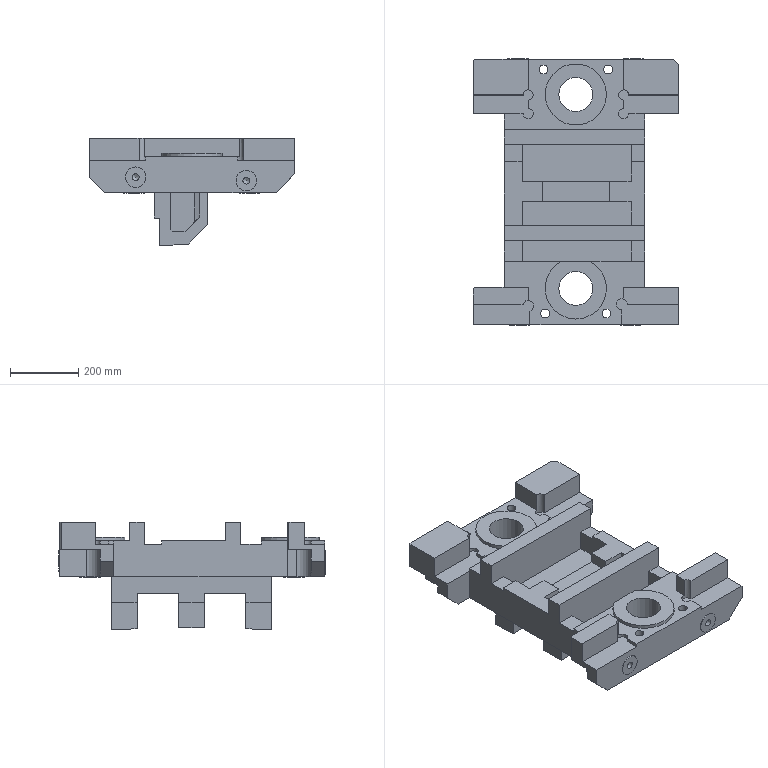Part | NX | features MAIN_BODY 2 | 1 solid | 210 faces | box 605 x 784 x 317.001 mm | volume 38669416 mm3 | plane 157 | cylinder 40 | cone 8 | spline 5 | commonest cylinder face diameters 20 x8 60 x8 26 x4 30 x4 41 x4 85 x4